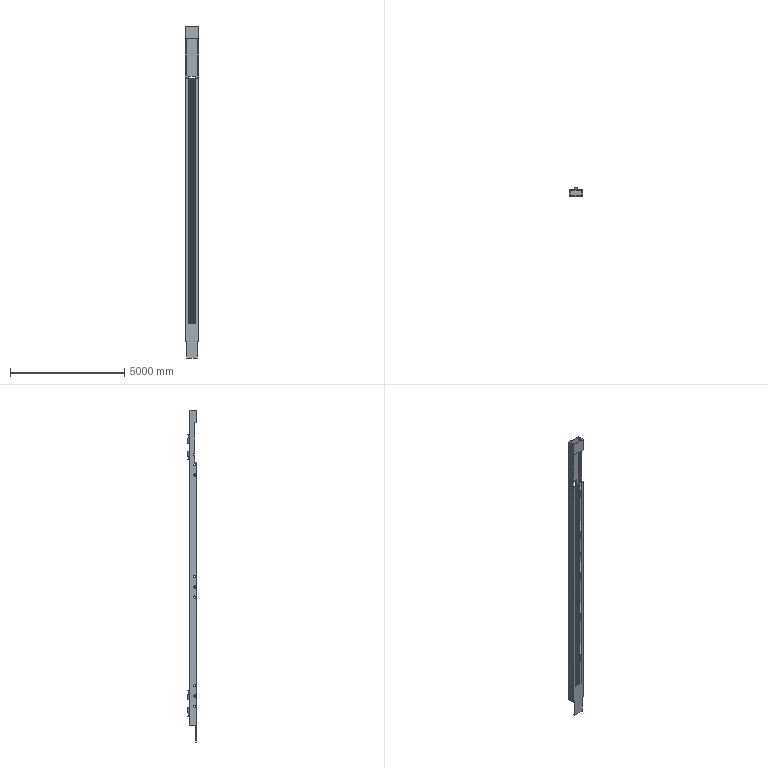Part | SolidWorks | features ICE 18, Extrusion 1 | 2 solids | 945 faces | box 600 x 410.622 x 14546 mm | volume 1021826260 mm3 | plane 893 | cylinder 52 | commonest cylinder face diameters 110 x28 69.032 x8 115.01 x6 134.27 x4 104.229 x3 116.312 x3